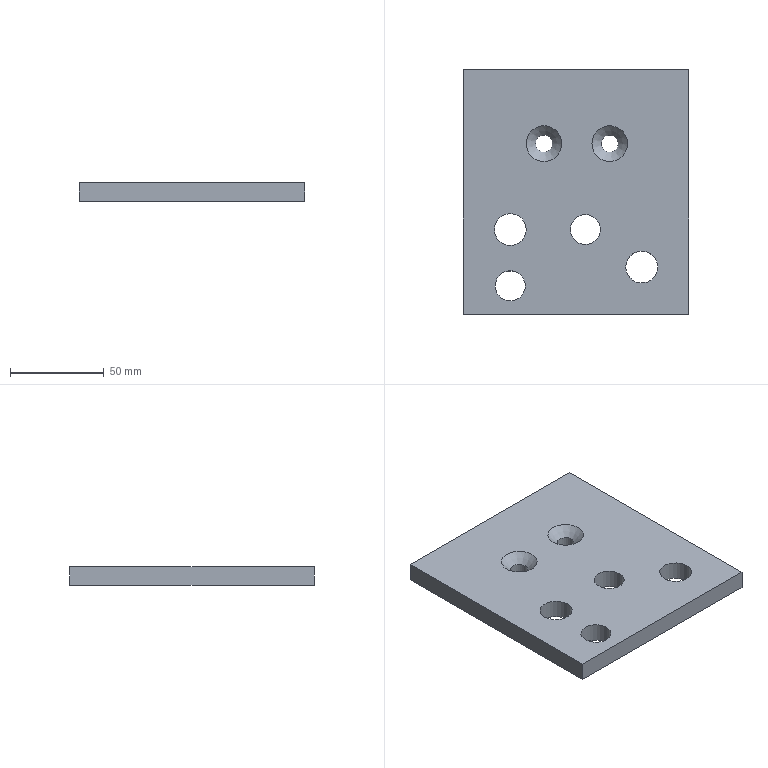Part | NX | features solid 2 | 1 solid | 14 faces | box 120 x 130 x 10 mm | volume 145198 mm3 | plane 6 | cylinder 6 | cone 2 | commonest cylinder face diameters 9 x2 16 x2 17 x2
STEP:
#1=CARTESIAN_POINT('',(-297.555,770.71,180.));
#2=VERTEX_POINT('',#1);
#3=CARTESIAN_POINT('',(-302.055,770.71,180.));
#4=DIRECTION('',(0.,0.,1.));
#5=DIRECTION('',(1.,0.,0.));
#6=AXIS2_PLACEMENT_3D('',#3,#4,#5);
#7=CIRCLE('',#6,4.5);
#8=EDGE_CURVE('',#2,#2,#7,.T.);
#9=ORIENTED_EDGE('',*,*,#8,.T.);
#10=EDGE_LOOP('',(#9));
#11=FACE_BOUND('',#10,.T.);
#12=CARTESIAN_POINT('',(-328.,695.,180.));
#13=VERTEX_POINT('',#12);
#14=CARTESIAN_POINT('',(-320.,695.,180.));
#15=DIRECTION('',(0.,0.,-1.));
#16=DIRECTION('',(-1.,0.,0.));
#17=AXIS2_PLACEMENT_3D('',#14,#15,#16);
#18=CIRCLE('',#17,8.);
#19=EDGE_CURVE('',#13,#13,#18,.T.);
#20=ORIENTED_EDGE('',*,*,#19,.F.);
#21=EDGE_LOOP('',(#20));
#22=FACE_BOUND('',#21,.T.);
#23=CARTESIAN_POINT('',(-241.5,705.,180.));
#24=VERTEX_POINT('',#23);
#25=CARTESIAN_POINT('',(-250.,705.,180.));
#26=DIRECTION('',(0.,0.,1.));
#27=DIRECTION('',(1.,0.,0.));
#28=AXIS2_PLACEMENT_3D('',#25,#26,#27);
#29=CIRCLE('',#28,8.5);
#30=EDGE_CURVE('',#24,#24,#29,.T.);
#31=ORIENTED_EDGE('',*,*,#30,.T.);
#32=EDGE_LOOP('',(#31));
#33=FACE_BOUND('',#32,.T.);
#34=CARTESIAN_POINT('',(-288.,725.,180.));
#35=VERTEX_POINT('',#34);
#36=CARTESIAN_POINT('',(-280.,725.,180.));
#37=DIRECTION('',(0.,0.,-1.));
#38=DIRECTION('',(-1.,0.,0.));
#39=AXIS2_PLACEMENT_3D('',#36,#37,#38);
#40=CIRCLE('',#39,8.);
#41=EDGE_CURVE('',#35,#35,#40,.T.);
#42=ORIENTED_EDGE('',*,*,#41,.F.);
#43=EDGE_LOOP('',(#42));
#44=FACE_BOUND('',#43,.T.);
#45=CARTESIAN_POINT('',(-225.,680.,180.));
#46=VERTEX_POINT('',#45);
#47=CARTESIAN_POINT('',(-225.,810.,180.));
#48=VERTEX_POINT('',#47);
#49=CARTESIAN_POINT('',(-225.,680.,180.));
#50=DIRECTION('',(0.,1.,0.));
#51=VECTOR('',#50,1000.);
#52=LINE('',#49,#51);
#53=EDGE_CURVE('',#46,#48,#52,.T.);
#54=ORIENTED_EDGE('',*,*,#53,.F.);
#55=CARTESIAN_POINT('',(-345.,680.,180.));
#56=VERTEX_POINT('',#55);
#57=CARTESIAN_POINT('',(-385.,680.,180.));
#58=DIRECTION('',(1.,0.,0.));
#59=VECTOR('',#58,1000.);
#60=LINE('',#57,#59);
#61=EDGE_CURVE('',#56,#46,#60,.T.);
#62=ORIENTED_EDGE('',*,*,#61,.F.);
#63=CARTESIAN_POINT('',(-345.,810.,180.));
#64=VERTEX_POINT('',#63);
#65=CARTESIAN_POINT('',(-345.,810.,180.));
#66=DIRECTION('',(0.,1.,0.));
#67=VECTOR('',#66,1000.);
#68=LINE('',#65,#67);
#69=EDGE_CURVE('',#56,#64,#68,.T.);
#70=ORIENTED_EDGE('',*,*,#69,.T.);
#71=CARTESIAN_POINT('',(-385.,810.,180.));
#72=DIRECTION('',(1.,0.,0.));
#73=VECTOR('',#72,1000.);
#74=LINE('',#71,#73);
#75=EDGE_CURVE('',#64,#48,#74,.T.);
#76=ORIENTED_EDGE('',*,*,#75,.T.);
#77=EDGE_LOOP('',(#54,#62,#70,#76));
#78=FACE_BOUND('',#77,.T.);
#79=CARTESIAN_POINT('',(-311.5,725.,180.));
#80=VERTEX_POINT('',#79);
#81=CARTESIAN_POINT('',(-320.,725.,180.));
#82=DIRECTION('',(0.,0.,1.));
#83=DIRECTION('',(1.,0.,0.));
#84=AXIS2_PLACEMENT_3D('',#81,#82,#83);
#85=CIRCLE('',#84,8.5);
#86=EDGE_CURVE('',#80,#80,#85,.T.);
#87=ORIENTED_EDGE('',*,*,#86,.T.);
#88=EDGE_LOOP('',(#87));
#89=FACE_BOUND('',#88,.T.);
#90=CARTESIAN_POINT('',(-262.544,770.71,180.));
#91=VERTEX_POINT('',#90);
#92=CARTESIAN_POINT('',(-267.044,770.71,180.));
#93=DIRECTION('',(0.,0.,1.));
#94=DIRECTION('',(1.,0.,0.));
#95=AXIS2_PLACEMENT_3D('',#92,#93,#94);
#96=CIRCLE('',#95,4.5);
#97=EDGE_CURVE('',#91,#91,#96,.T.);
#98=ORIENTED_EDGE('',*,*,#97,.T.);
#99=EDGE_LOOP('',(#98));
#100=FACE_BOUND('',#99,.T.);
#101=CARTESIAN_POINT('',(-225.,810.,180.));
#102=DIRECTION('',(0.,0.,-1.));
#103=DIRECTION('',(0.,1.,0.));
#104=AXIS2_PLACEMENT_3D('',#101,#102,#103);
#105=PLANE('',#104);
#106=ADVANCED_FACE('',(#11,#22,#33,#44,#78,#89,#100),#105,.T.);
#107=CARTESIAN_POINT('',(-292.555,770.71,190.));
#108=VERTEX_POINT('',#107);
#109=CARTESIAN_POINT('',(-302.055,770.71,190.));
#110=DIRECTION('',(0.,0.,1.));
#111=DIRECTION('',(1.,0.,0.));
#112=AXIS2_PLACEMENT_3D('',#109,#110,#111);
#113=CIRCLE('',#112,9.5);
#114=EDGE_CURVE('',#108,#108,#113,.T.);
#115=ORIENTED_EDGE('',*,*,#114,.F.);
#116=EDGE_LOOP('',(#115));
#117=FACE_BOUND('',#116,.T.);
#118=CARTESIAN_POINT('',(-257.544,770.71,190.));
#119=VERTEX_POINT('',#118);
#120=CARTESIAN_POINT('',(-267.044,770.71,190.));
#121=DIRECTION('',(0.,0.,1.));
#122=DIRECTION('',(1.,0.,0.));
#123=AXIS2_PLACEMENT_3D('',#120,#121,#122);
#124=CIRCLE('',#123,9.5);
#125=EDGE_CURVE('',#119,#119,#124,.T.);
#126=ORIENTED_EDGE('',*,*,#125,.F.);
#127=EDGE_LOOP('',(#126));
#128=FACE_BOUND('',#127,.T.);
#129=CARTESIAN_POINT('',(-328.,695.,190.));
#130=VERTEX_POINT('',#129);
#131=CARTESIAN_POINT('',(-320.,695.,190.));
#132=DIRECTION('',(0.,0.,-1.));
#133=DIRECTION('',(-1.,0.,0.));
#134=AXIS2_PLACEMENT_3D('',#131,#132,#133);
#135=CIRCLE('',#134,8.);
#136=EDGE_CURVE('',#130,#130,#135,.T.);
#137=ORIENTED_EDGE('',*,*,#136,.T.);
#138=EDGE_LOOP('',(#137));
#139=FACE_BOUND('',#138,.T.);
#140=CARTESIAN_POINT('',(-258.5,705.,190.));
#141=VERTEX_POINT('',#140);
#142=CARTESIAN_POINT('',(-250.,705.,190.));
#143=DIRECTION('',(0.,0.,-1.));
#144=DIRECTION('',(-1.,0.,0.));
#145=AXIS2_PLACEMENT_3D('',#142,#143,#144);
#146=CIRCLE('',#145,8.5);
#147=EDGE_CURVE('',#141,#141,#146,.F.);
#148=ORIENTED_EDGE('',*,*,#147,.F.);
#149=EDGE_LOOP('',(#148));
#150=FACE_BOUND('',#149,.T.);
#151=CARTESIAN_POINT('',(-288.,725.,190.));
#152=VERTEX_POINT('',#151);
#153=CARTESIAN_POINT('',(-280.,725.,190.));
#154=DIRECTION('',(0.,0.,-1.));
#155=DIRECTION('',(-1.,0.,0.));
#156=AXIS2_PLACEMENT_3D('',#153,#154,#155);
#157=CIRCLE('',#156,8.);
#158=EDGE_CURVE('',#152,#152,#157,.T.);
#159=ORIENTED_EDGE('',*,*,#158,.T.);
#160=EDGE_LOOP('',(#159));
#161=FACE_BOUND('',#160,.T.);
#162=CARTESIAN_POINT('',(-225.,680.,190.));
#163=VERTEX_POINT('',#162);
#164=CARTESIAN_POINT('',(-225.,810.,190.));
#165=VERTEX_POINT('',#164);
#166=CARTESIAN_POINT('',(-225.,810.,190.));
#167=DIRECTION('',(0.,1.,0.));
#168=VECTOR('',#167,1000.);
#169=LINE('',#166,#168);
#170=EDGE_CURVE('',#163,#165,#169,.T.);
#171=ORIENTED_EDGE('',*,*,#170,.T.);
#172=CARTESIAN_POINT('',(-345.,810.,190.));
#173=VERTEX_POINT('',#172);
#174=CARTESIAN_POINT('',(-225.,810.,190.));
#175=DIRECTION('',(1.,0.,0.));
#176=VECTOR('',#175,1000.);
#177=LINE('',#174,#176);
#178=EDGE_CURVE('',#173,#165,#177,.T.);
#179=ORIENTED_EDGE('',*,*,#178,.F.);
#180=CARTESIAN_POINT('',(-345.,680.,190.));
#181=VERTEX_POINT('',#180);
#182=CARTESIAN_POINT('',(-345.,810.,190.));
#183=DIRECTION('',(0.,1.,0.));
#184=VECTOR('',#183,1000.);
#185=LINE('',#182,#184);
#186=EDGE_CURVE('',#181,#173,#185,.T.);
#187=ORIENTED_EDGE('',*,*,#186,.F.);
#188=CARTESIAN_POINT('',(-225.,680.,190.));
#189=DIRECTION('',(1.,0.,0.));
#190=VECTOR('',#189,1000.);
#191=LINE('',#188,#190);
#192=EDGE_CURVE('',#181,#163,#191,.T.);
#193=ORIENTED_EDGE('',*,*,#192,.T.);
#194=EDGE_LOOP('',(#171,#179,#187,#193));
#195=FACE_BOUND('',#194,.T.);
#196=CARTESIAN_POINT('',(-328.5,725.,190.));
#197=VERTEX_POINT('',#196);
#198=CARTESIAN_POINT('',(-320.,725.,190.));
#199=DIRECTION('',(0.,0.,-1.));
#200=DIRECTION('',(-1.,0.,0.));
#201=AXIS2_PLACEMENT_3D('',#198,#199,#200);
#202=CIRCLE('',#201,8.5);
#203=EDGE_CURVE('',#197,#197,#202,.F.);
#204=ORIENTED_EDGE('',*,*,#203,.F.);
#205=EDGE_LOOP('',(#204));
#206=FACE_BOUND('',#205,.T.);
#207=CARTESIAN_POINT('',(-225.,810.,190.));
#208=DIRECTION('',(0.,0.,-1.));
#209=DIRECTION('',(0.,1.,0.));
#210=AXIS2_PLACEMENT_3D('',#207,#208,#209);
#211=PLANE('',#210);
#212=ADVANCED_FACE('',(#117,#128,#139,#150,#161,#195,#206),#211,.F.);
#213=ORIENTED_EDGE('',*,*,#53,.T.);
#214=CARTESIAN_POINT('',(-225.,810.,185.));
#215=DIRECTION('',(0.,0.,-1.));
#216=VECTOR('',#215,1000.);
#217=LINE('',#214,#216);
#218=EDGE_CURVE('',#165,#48,#217,.T.);
#219=ORIENTED_EDGE('',*,*,#218,.F.);
#220=ORIENTED_EDGE('',*,*,#170,.F.);
#221=CARTESIAN_POINT('',(-225.,680.,185.));
#222=DIRECTION('',(0.,0.,-1.));
#223=VECTOR('',#222,1000.);
#224=LINE('',#221,#223);
#225=EDGE_CURVE('',#163,#46,#224,.T.);
#226=ORIENTED_EDGE('',*,*,#225,.T.);
#227=EDGE_LOOP('',(#213,#219,#220,#226));
#228=FACE_BOUND('',#227,.T.);
#229=CARTESIAN_POINT('',(-225.,680.,185.));
#230=DIRECTION('',(-1.,0.,0.));
#231=DIRECTION('',(0.,0.,-1.));
#232=AXIS2_PLACEMENT_3D('',#229,#230,#231);
#233=PLANE('',#232);
#234=ADVANCED_FACE('',(#228),#233,.F.);
#235=ORIENTED_EDGE('',*,*,#75,.F.);
#236=CARTESIAN_POINT('',(-345.,810.,185.));
#237=DIRECTION('',(0.,0.,-1.));
#238=VECTOR('',#237,1000.);
#239=LINE('',#236,#238);
#240=EDGE_CURVE('',#173,#64,#239,.T.);
#241=ORIENTED_EDGE('',*,*,#240,.F.);
#242=ORIENTED_EDGE('',*,*,#178,.T.);
#243=ORIENTED_EDGE('',*,*,#218,.T.);
#244=EDGE_LOOP('',(#235,#241,#242,#243));
#245=FACE_BOUND('',#244,.T.);
#246=CARTESIAN_POINT('',(-385.,810.,185.));
#247=DIRECTION('',(0.,1.,0.));
#248=DIRECTION('',(-1.,0.,0.));
#249=AXIS2_PLACEMENT_3D('',#246,#247,#248);
#250=PLANE('',#249);
#251=ADVANCED_FACE('',(#245),#250,.T.);
#252=ORIENTED_EDGE('',*,*,#69,.F.);
#253=CARTESIAN_POINT('',(-345.,680.,185.));
#254=DIRECTION('',(0.,0.,-1.));
#255=VECTOR('',#254,1000.);
#256=LINE('',#253,#255);
#257=EDGE_CURVE('',#181,#56,#256,.T.);
#258=ORIENTED_EDGE('',*,*,#257,.F.);
#259=ORIENTED_EDGE('',*,*,#186,.T.);
#260=ORIENTED_EDGE('',*,*,#240,.T.);
#261=EDGE_LOOP('',(#252,#258,#259,#260));
#262=FACE_BOUND('',#261,.T.);
#263=CARTESIAN_POINT('',(-345.,680.,185.));
#264=DIRECTION('',(-1.,0.,0.));
#265=DIRECTION('',(0.,0.,-1.));
#266=AXIS2_PLACEMENT_3D('',#263,#264,#265);
#267=PLANE('',#266);
#268=ADVANCED_FACE('',(#262),#267,.T.);
#269=ORIENTED_EDGE('',*,*,#61,.T.);
#270=ORIENTED_EDGE('',*,*,#225,.F.);
#271=ORIENTED_EDGE('',*,*,#192,.F.);
#272=ORIENTED_EDGE('',*,*,#257,.T.);
#273=EDGE_LOOP('',(#269,#270,#271,#272));
#274=FACE_BOUND('',#273,.T.);
#275=CARTESIAN_POINT('',(-385.,680.,185.));
#276=DIRECTION('',(0.,1.,0.));
#277=DIRECTION('',(-1.,0.,0.));
#278=AXIS2_PLACEMENT_3D('',#275,#276,#277);
#279=PLANE('',#278);
#280=ADVANCED_FACE('',(#274),#279,.F.);
#281=ORIENTED_EDGE('',*,*,#203,.T.);
#282=EDGE_LOOP('',(#281));
#283=FACE_BOUND('',#282,.T.);
#284=ORIENTED_EDGE('',*,*,#86,.F.);
#285=EDGE_LOOP('',(#284));
#286=FACE_BOUND('',#285,.T.);
#287=CARTESIAN_POINT('',(-320.,725.,185.));
#288=DIRECTION('',(0.,0.,-1.));
#289=DIRECTION('',(-1.,0.,0.));
#290=AXIS2_PLACEMENT_3D('',#287,#288,#289);
#291=CYLINDRICAL_SURFACE('',#290,8.5);
#292=ADVANCED_FACE('',(#283,#286),#291,.F.);
#293=ORIENTED_EDGE('',*,*,#158,.F.);
#294=EDGE_LOOP('',(#293));
#295=FACE_BOUND('',#294,.T.);
#296=ORIENTED_EDGE('',*,*,#41,.T.);
#297=EDGE_LOOP('',(#296));
#298=FACE_BOUND('',#297,.T.);
#299=CARTESIAN_POINT('',(-280.,725.,185.));
#300=DIRECTION('',(0.,0.,-1.));
#301=DIRECTION('',(-1.,0.,0.));
#302=AXIS2_PLACEMENT_3D('',#299,#300,#301);
#303=CYLINDRICAL_SURFACE('',#302,8.);
#304=ADVANCED_FACE('',(#295,#298),#303,.F.);
#305=ORIENTED_EDGE('',*,*,#147,.T.);
#306=EDGE_LOOP('',(#305));
#307=FACE_BOUND('',#306,.T.);
#308=ORIENTED_EDGE('',*,*,#30,.F.);
#309=EDGE_LOOP('',(#308));
#310=FACE_BOUND('',#309,.T.);
#311=CARTESIAN_POINT('',(-250.,705.,185.));
#312=DIRECTION('',(0.,0.,-1.));
#313=DIRECTION('',(-1.,0.,0.));
#314=AXIS2_PLACEMENT_3D('',#311,#312,#313);
#315=CYLINDRICAL_SURFACE('',#314,8.5);
#316=ADVANCED_FACE('',(#307,#310),#315,.F.);
#317=ORIENTED_EDGE('',*,*,#19,.T.);
#318=EDGE_LOOP('',(#317));
#319=FACE_BOUND('',#318,.T.);
#320=ORIENTED_EDGE('',*,*,#136,.F.);
#321=EDGE_LOOP('',(#320));
#322=FACE_BOUND('',#321,.T.);
#323=CARTESIAN_POINT('',(-320.,695.,150.));
#324=DIRECTION('',(0.,0.,1.));
#325=DIRECTION('',(1.,0.,0.));
#326=AXIS2_PLACEMENT_3D('',#323,#324,#325);
#327=CYLINDRICAL_SURFACE('',#326,8.);
#328=ADVANCED_FACE('',(#319,#322),#327,.F.);
#329=CARTESIAN_POINT('',(-262.544,770.71,185.));
#330=VERTEX_POINT('',#329);
#331=CARTESIAN_POINT('',(-267.044,770.71,185.));
#332=DIRECTION('',(0.,0.,1.));
#333=DIRECTION('',(1.,0.,0.));
#334=AXIS2_PLACEMENT_3D('',#331,#332,#333);
#335=CIRCLE('',#334,4.5);
#336=EDGE_CURVE('',#330,#330,#335,.T.);
#337=ORIENTED_EDGE('',*,*,#336,.F.);
#338=EDGE_LOOP('',(#337));
#339=FACE_BOUND('',#338,.T.);
#340=ORIENTED_EDGE('',*,*,#125,.T.);
#341=EDGE_LOOP('',(#340));
#342=FACE_BOUND('',#341,.T.);
#343=CARTESIAN_POINT('',(-267.044,770.71,190.));
#344=DIRECTION('',(0.,0.,1.));
#345=DIRECTION('',(1.,0.,0.));
#346=AXIS2_PLACEMENT_3D('',#343,#344,#345);
#347=CONICAL_SURFACE('',#346,9.5,0.7854);
#348=ADVANCED_FACE('',(#339,#342),#347,.F.);
#349=CARTESIAN_POINT('',(-297.555,770.71,185.));
#350=VERTEX_POINT('',#349);
#351=CARTESIAN_POINT('',(-302.055,770.71,185.));
#352=DIRECTION('',(0.,0.,1.));
#353=DIRECTION('',(1.,0.,0.));
#354=AXIS2_PLACEMENT_3D('',#351,#352,#353);
#355=CIRCLE('',#354,4.5);
#356=EDGE_CURVE('',#350,#350,#355,.T.);
#357=ORIENTED_EDGE('',*,*,#356,.F.);
#358=EDGE_LOOP('',(#357));
#359=FACE_BOUND('',#358,.T.);
#360=ORIENTED_EDGE('',*,*,#114,.T.);
#361=EDGE_LOOP('',(#360));
#362=FACE_BOUND('',#361,.T.);
#363=CARTESIAN_POINT('',(-302.055,770.71,190.));
#364=DIRECTION('',(0.,0.,1.));
#365=DIRECTION('',(1.,0.,0.));
#366=AXIS2_PLACEMENT_3D('',#363,#364,#365);
#367=CONICAL_SURFACE('',#366,9.5,0.7854);
#368=ADVANCED_FACE('',(#359,#362),#367,.F.);
#369=ORIENTED_EDGE('',*,*,#356,.T.);
#370=EDGE_LOOP('',(#369));
#371=FACE_BOUND('',#370,.T.);
#372=ORIENTED_EDGE('',*,*,#8,.F.);
#373=EDGE_LOOP('',(#372));
#374=FACE_BOUND('',#373,.T.);
#375=CARTESIAN_POINT('',(-302.055,770.71,185.));
#376=DIRECTION('',(0.,0.,-1.));
#377=DIRECTION('',(-1.,0.,0.));
#378=AXIS2_PLACEMENT_3D('',#375,#376,#377);
#379=CYLINDRICAL_SURFACE('',#378,4.5);
#380=ADVANCED_FACE('',(#371,#374),#379,.F.);
#381=ORIENTED_EDGE('',*,*,#336,.T.);
#382=EDGE_LOOP('',(#381));
#383=FACE_BOUND('',#382,.T.);
#384=ORIENTED_EDGE('',*,*,#97,.F.);
#385=EDGE_LOOP('',(#384));
#386=FACE_BOUND('',#385,.T.);
#387=CARTESIAN_POINT('',(-267.044,770.71,185.));
#388=DIRECTION('',(0.,0.,-1.));
#389=DIRECTION('',(-1.,0.,0.));
#390=AXIS2_PLACEMENT_3D('',#387,#388,#389);
#391=CYLINDRICAL_SURFACE('',#390,4.5);
#392=ADVANCED_FACE('',(#383,#386),#391,.F.);
#393=CLOSED_SHELL('',(#106,#212,#234,#251,#268,#280,#292,#304,#316,#328,#348,#368,#380,#392));
#394=MANIFOLD_SOLID_BREP('',#393);
#395=(LENGTH_UNIT()NAMED_UNIT(*)SI_UNIT(.MILLI.,.METRE.));
#396=UNCERTAINTY_MEASURE_WITH_UNIT(LENGTH_MEASURE(0.00001),#395,'','');
#397=(NAMED_UNIT(*)PLANE_ANGLE_UNIT()SI_UNIT($,.RADIAN.));
#398=(NAMED_UNIT(*)SI_UNIT($,.STERADIAN.)SOLID_ANGLE_UNIT());
#399=(GEOMETRIC_REPRESENTATION_CONTEXT(3)GLOBAL_UNCERTAINTY_ASSIGNED_CONTEXT((#396))GLOBAL_UNIT_ASSIGNED_CONTEXT((#395,#397,#398))REPRESENTATION_CONTEXT('',''));
#400=ADVANCED_BREP_SHAPE_REPRESENTATION('',(#394),#399);